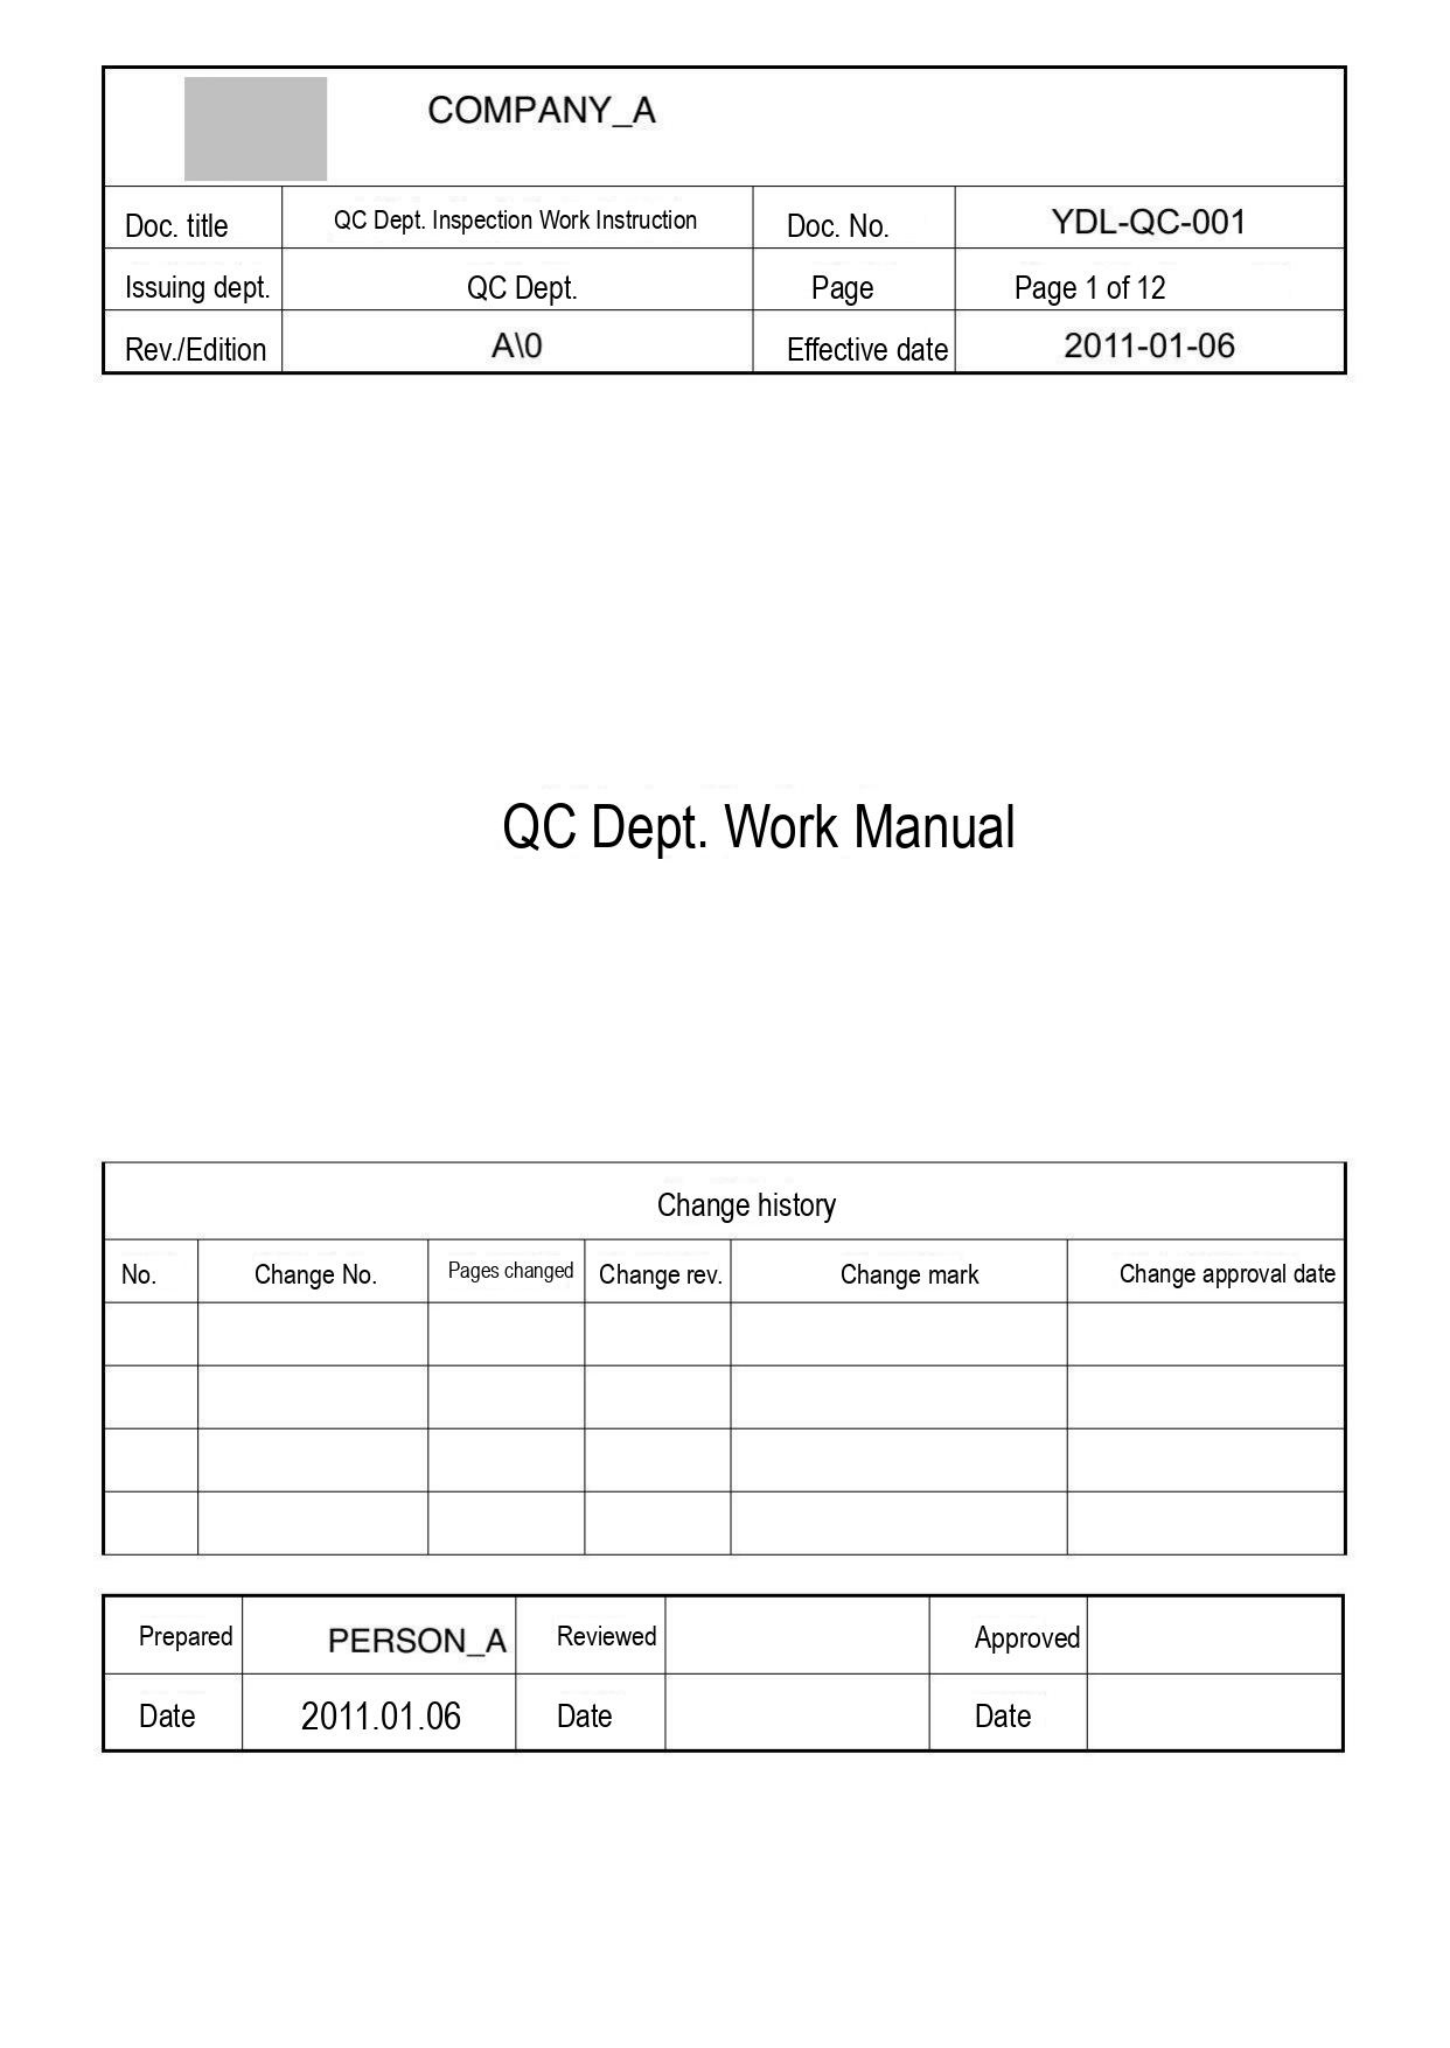COMPANY_A

| Doc. title | QC Dept. Inspection Work Instruction | Doc. No. | YDL-QC-001 |
|---|---|---|---|
| Issuing dept. | QC Dept. | Page | Page 1 of 12 |
| Rev./Edition | A\0 | Effective date | 2011-01-06 |

QC Dept. Work Manual

Change history

| No. | Change No. | Pages changed | Change rev. | Change mark | Change approval date |
|---|---|---|---|---|---|
| | | | | | |
| | | | | | |
| | | | | | |
| | | | | | |

| Prepared | PERSON_A | Reviewed | | Approved | |
|---|---|---|---|---|---|
| Date | 2011.01.06 | Date | | Date | |
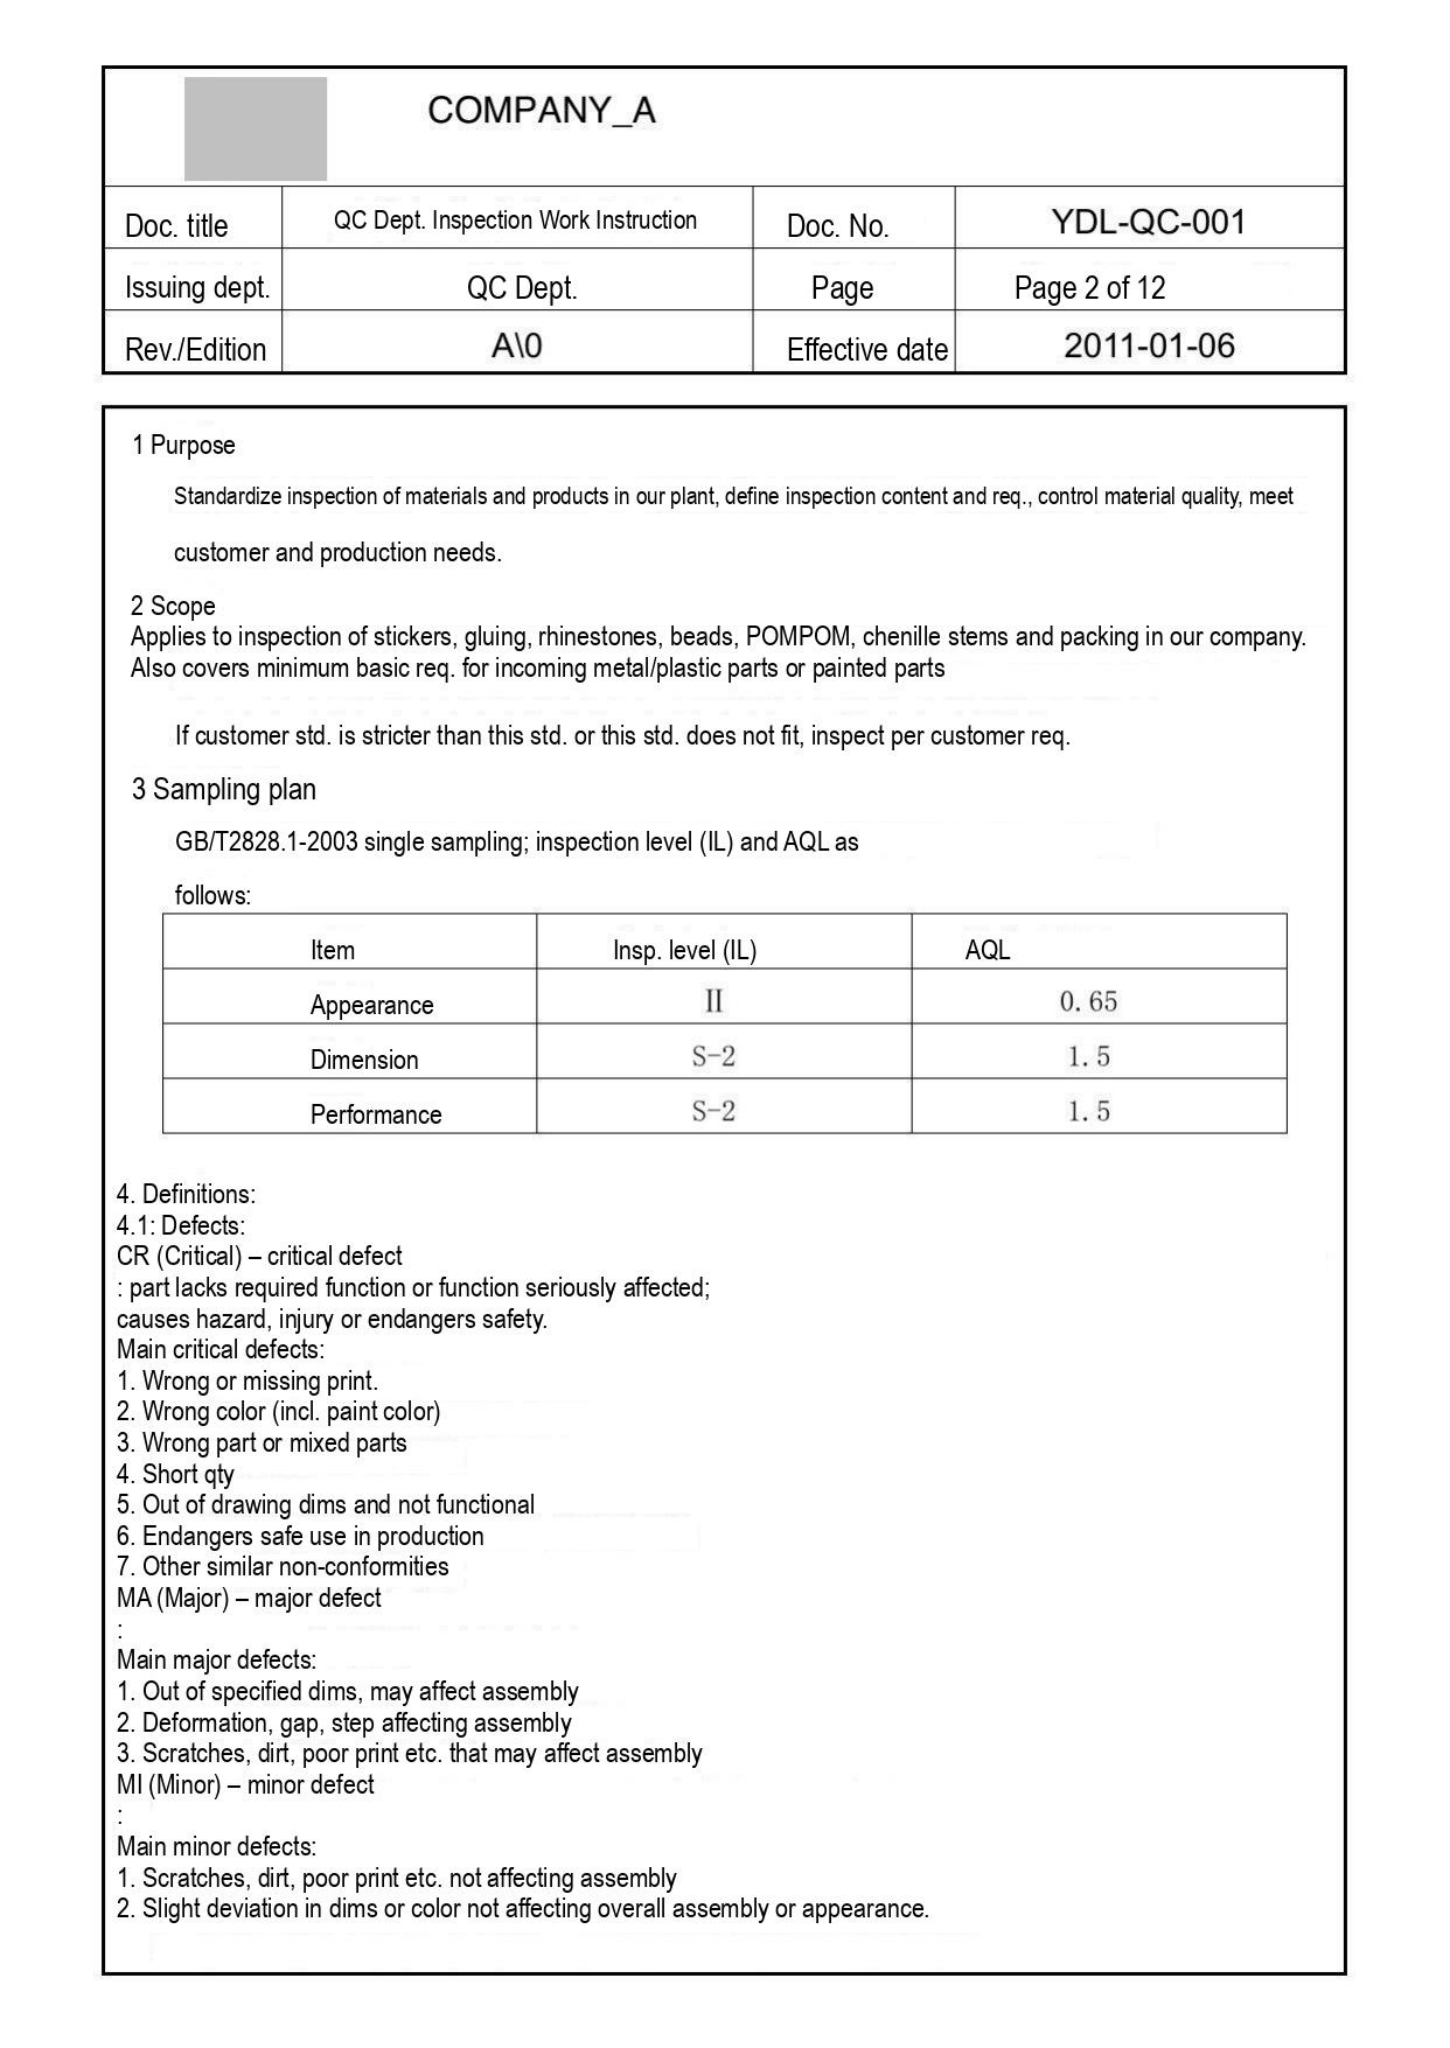COMPANY_A

| Doc. title | QC Dept. Inspection Work Instruction | Doc. No. | YDL-QC-001 |
|---|---|---|---|
| Issuing dept. | QC Dept. | Page | Page 2 of 12 |
| Rev./Edition | A\0 | Effective date | 2011-01-06 |

1 Purpose

Standardize inspection of materials and products in our plant, define inspection content and req., control material quality, meet customer and production needs.

2 Scope
Applies to inspection of stickers, gluing, rhinestones, beads, POMPOM, chenille stems and packing in our company. Also covers minimum basic req. for incoming metal/plastic parts or painted parts

If customer std. is stricter than this std. or this std. does not fit, inspect per customer req.

3 Sampling plan

GB/T2828.1-2003 single sampling; inspection level (IL) and AQL as follows:

| Item | Insp. level (IL) | AQL |
|---|---|---|
| Appearance | II | 0. 65 |
| Dimension | S-2 | 1. 5 |
| Performance | S-2 | 1. 5 |

4. Definitions:
4.1: Defects:
CR (Critical) – critical defect
: part lacks required function or function seriously affected;
causes hazard, injury or endangers safety.
Main critical defects:
1. Wrong or missing print.
2. Wrong color (incl. paint color)
3. Wrong part or mixed parts
4. Short qty
5. Out of drawing dims and not functional
6. Endangers safe use in production
7. Other similar non-conformities
MA (Major) – major defect
:
Main major defects:
1. Out of specified dims, may affect assembly
2. Deformation, gap, step affecting assembly
3. Scratches, dirt, poor print etc. that may affect assembly
MI (Minor) – minor defect
:
Main minor defects:
1. Scratches, dirt, poor print etc. not affecting assembly
2. Slight deviation in dims or color not affecting overall assembly or appearance.
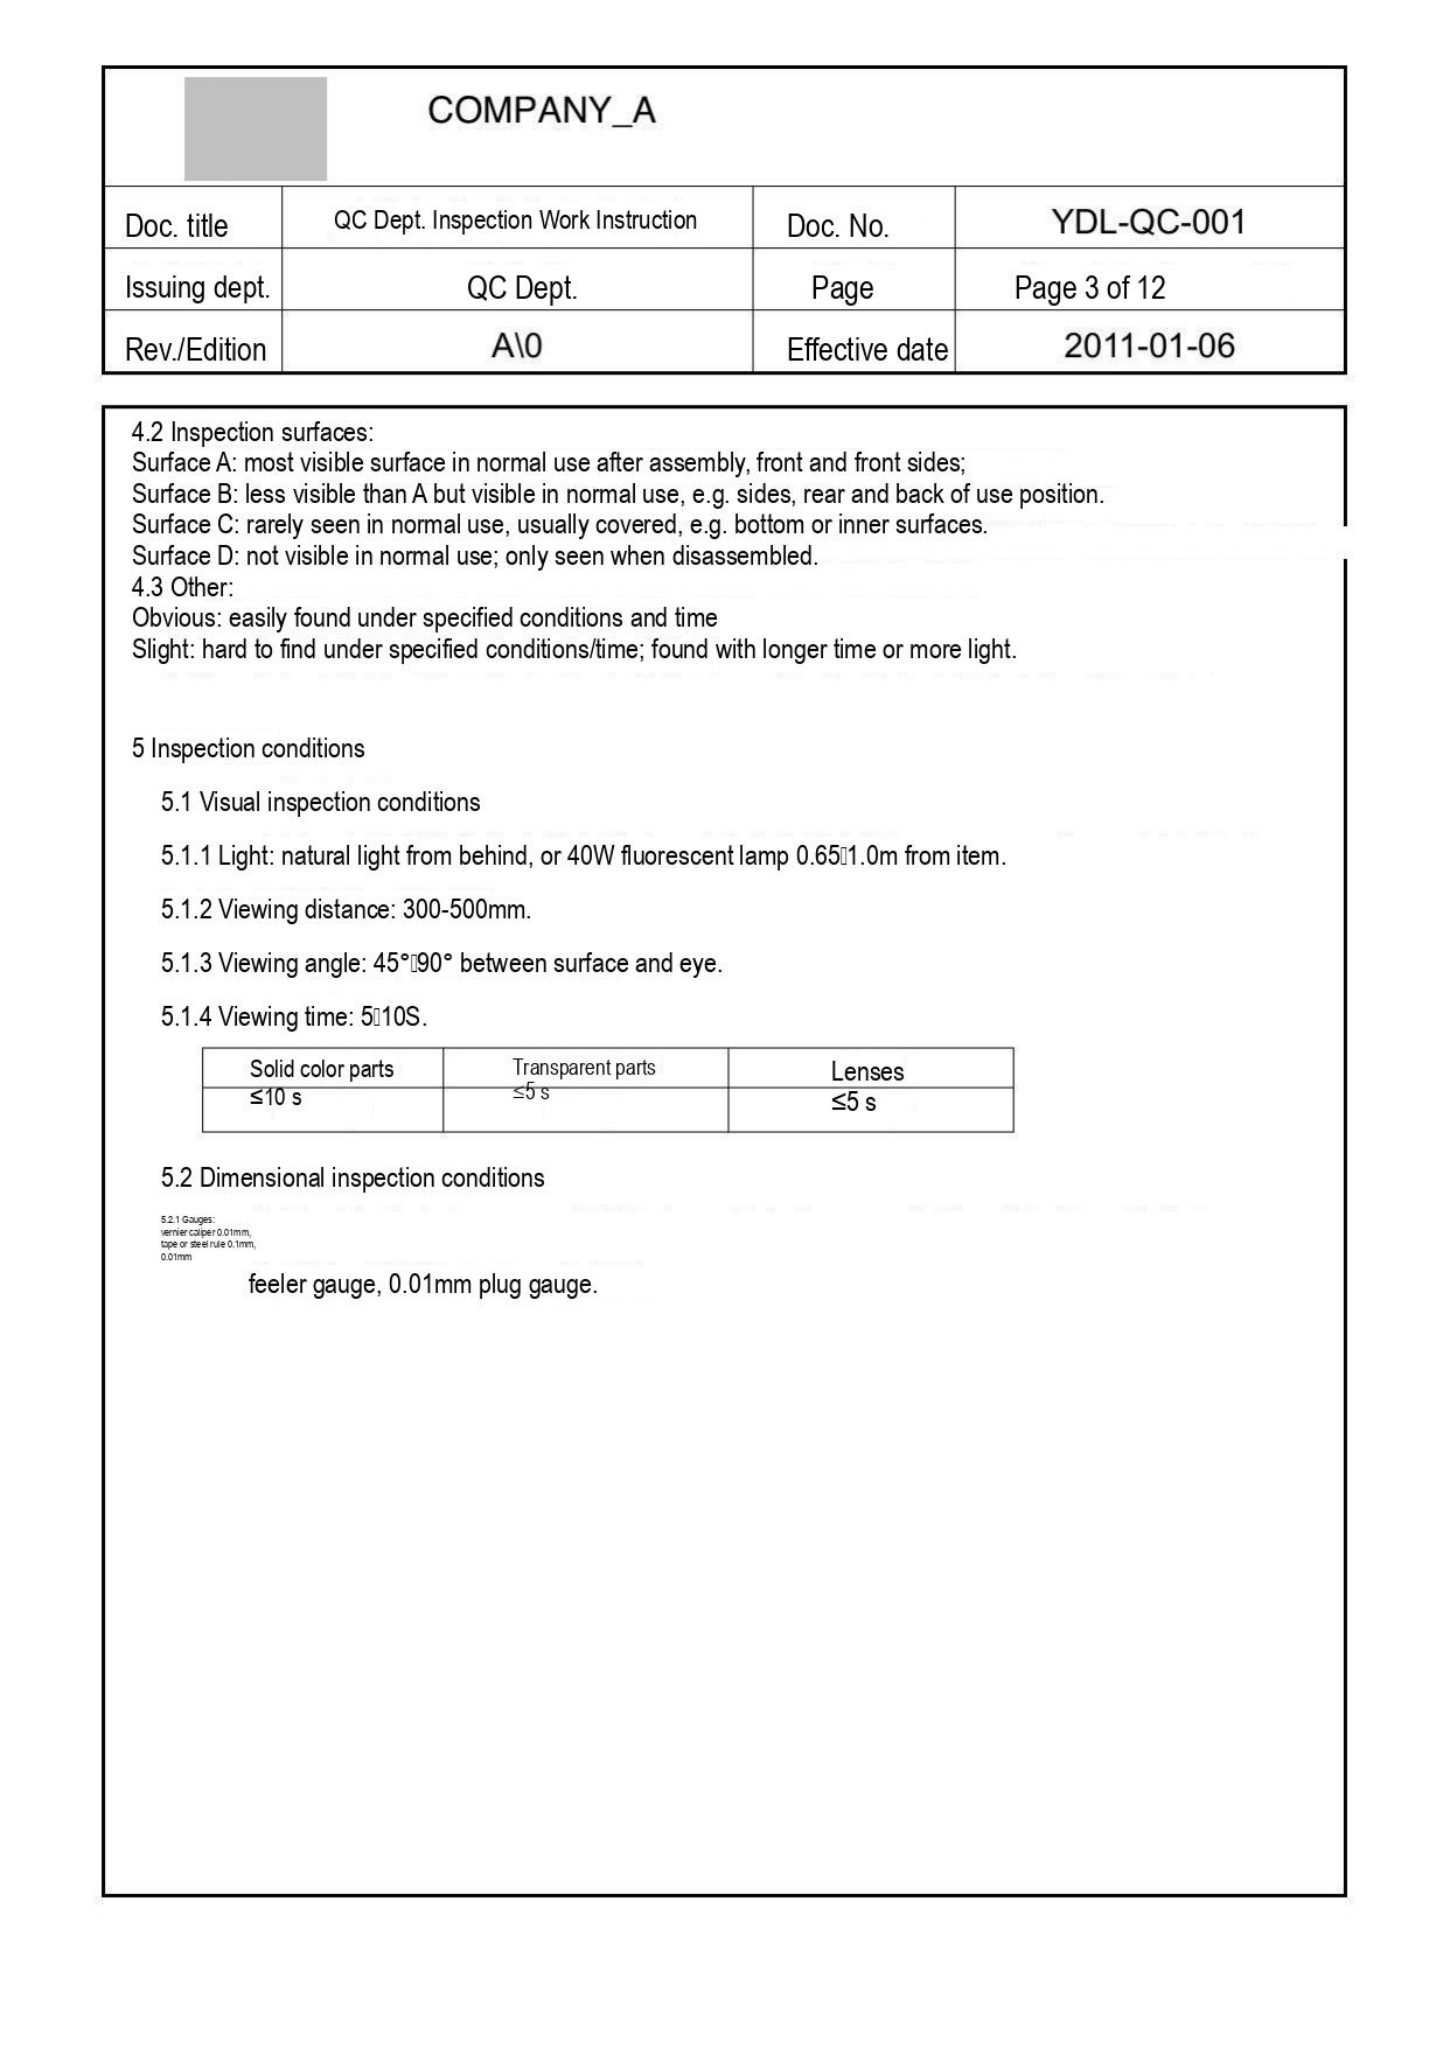COMPANY_A

| Doc. title | QC Dept. Inspection Work Instruction | Doc. No. | YDL-QC-001 |
|---|---|---|---|
| Issuing dept. | QC Dept. | Page | Page 3 of 12 |
| Rev./Edition | A\0 | Effective date | 2011-01-06 |

4.2 Inspection surfaces:
Surface A: most visible surface in normal use after assembly, front and front sides;
Surface B: less visible than A but visible in normal use, e.g. sides, rear and back of use position.
Surface C: rarely seen in normal use, usually covered, e.g. bottom or inner surfaces.
Surface D: not visible in normal use; only seen when disassembled.
4.3 Other:
Obvious: easily found under specified conditions and time
Slight: hard to find under specified conditions/time; found with longer time or more light.

5 Inspection conditions

5.1 Visual inspection conditions

5.1.1 Light: natural light from behind, or 40W fluorescent lamp 0.65 1.0m from item.

5.1.2 Viewing distance: 300-500mm.

5.1.3 Viewing angle: 45° 90° between surface and eye.

5.1.4 Viewing time: 5 10S.

| Solid color parts | Transparent parts | Lenses |
|---|---|---|
| ≤10 s | ≤5 s | ≤5 s |

5.2 Dimensional inspection conditions

5.2.1 Gauges:
vernier caliper 0.01mm,
tape or steel rule 0.1mm,
0.01mm

feeler gauge, 0.01mm plug gauge.
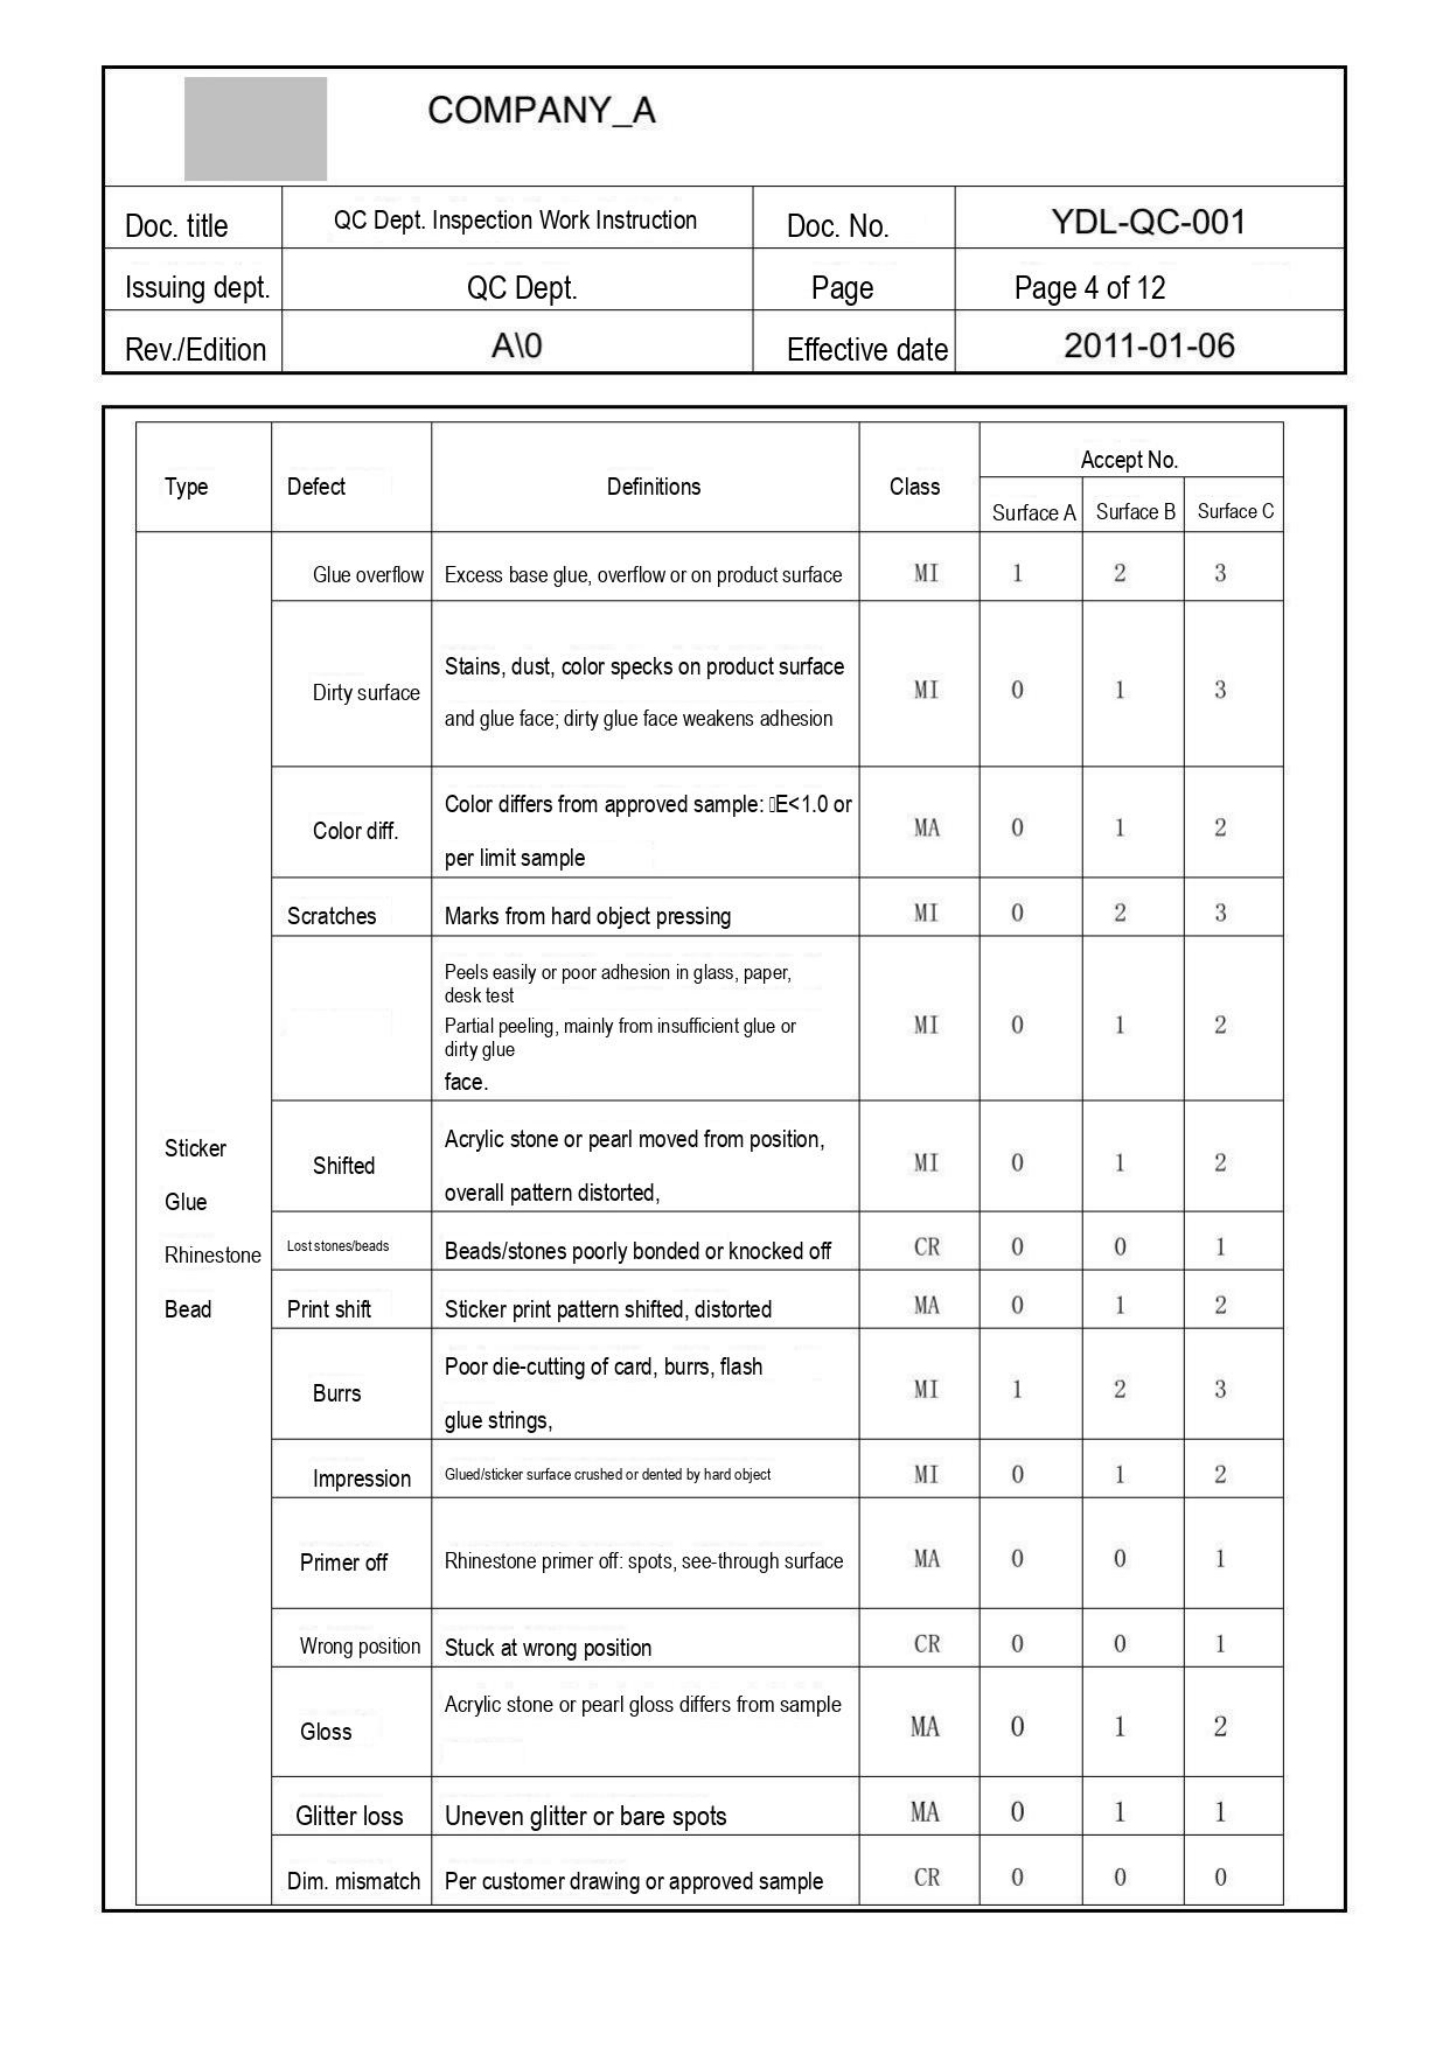COMPANY_A

| Doc. title | QC Dept. Inspection Work Instruction | Doc. No. | YDL-QC-001 |
|---|---|---|---|
| Issuing dept. | QC Dept. | Page | Page 4 of 12 |
| Rev./Edition | A\0 | Effective date | 2011-01-06 |

| Type | Defect | Definitions | Class | Accept No. Surface A | Accept No. Surface B | Accept No. Surface C |
|---|---|---|---|---|---|---|
| Sticker Glue Rhinestone Bead | Glue overflow | Excess base glue, overflow or on product surface | MI | 1 | 2 | 3 |
| | Dirty surface | Stains, dust, color specks on product surface and glue face; dirty glue face weakens adhesion | MI | 0 | 1 | 3 |
| | Color diff. | Color differs from approved sample: E<1.0 or per limit sample | MA | 0 | 1 | 2 |
| | Scratches | Marks from hard object pressing | MI | 0 | 2 | 3 |
| | | Peels easily or poor adhesion in glass, paper, desk test Partial peeling, mainly from insufficient glue or dirty glue face. | MI | 0 | 1 | 2 |
| | Shifted | Acrylic stone or pearl moved from position, overall pattern distorted, | MI | 0 | 1 | 2 |
| | Lost stones/beads | Beads/stones poorly bonded or knocked off | CR | 0 | 0 | 1 |
| | Print shift | Sticker print pattern shifted, distorted | MA | 0 | 1 | 2 |
| | Burrs | Poor die-cutting of card, burrs, flash glue strings, | MI | 1 | 2 | 3 |
| | Impression | Glued/sticker surface crushed or dented by hard object | MI | 0 | 1 | 2 |
| | Primer off | Rhinestone primer off: spots, see-through surface | MA | 0 | 0 | 1 |
| | Wrong position | Stuck at wrong position | CR | 0 | 0 | 1 |
| | Gloss | Acrylic stone or pearl gloss differs from sample | MA | 0 | 1 | 2 |
| | Glitter loss | Uneven glitter or bare spots | MA | 0 | 1 | 1 |
| | Dim. mismatch | Per customer drawing or approved sample | CR | 0 | 0 | 0 |
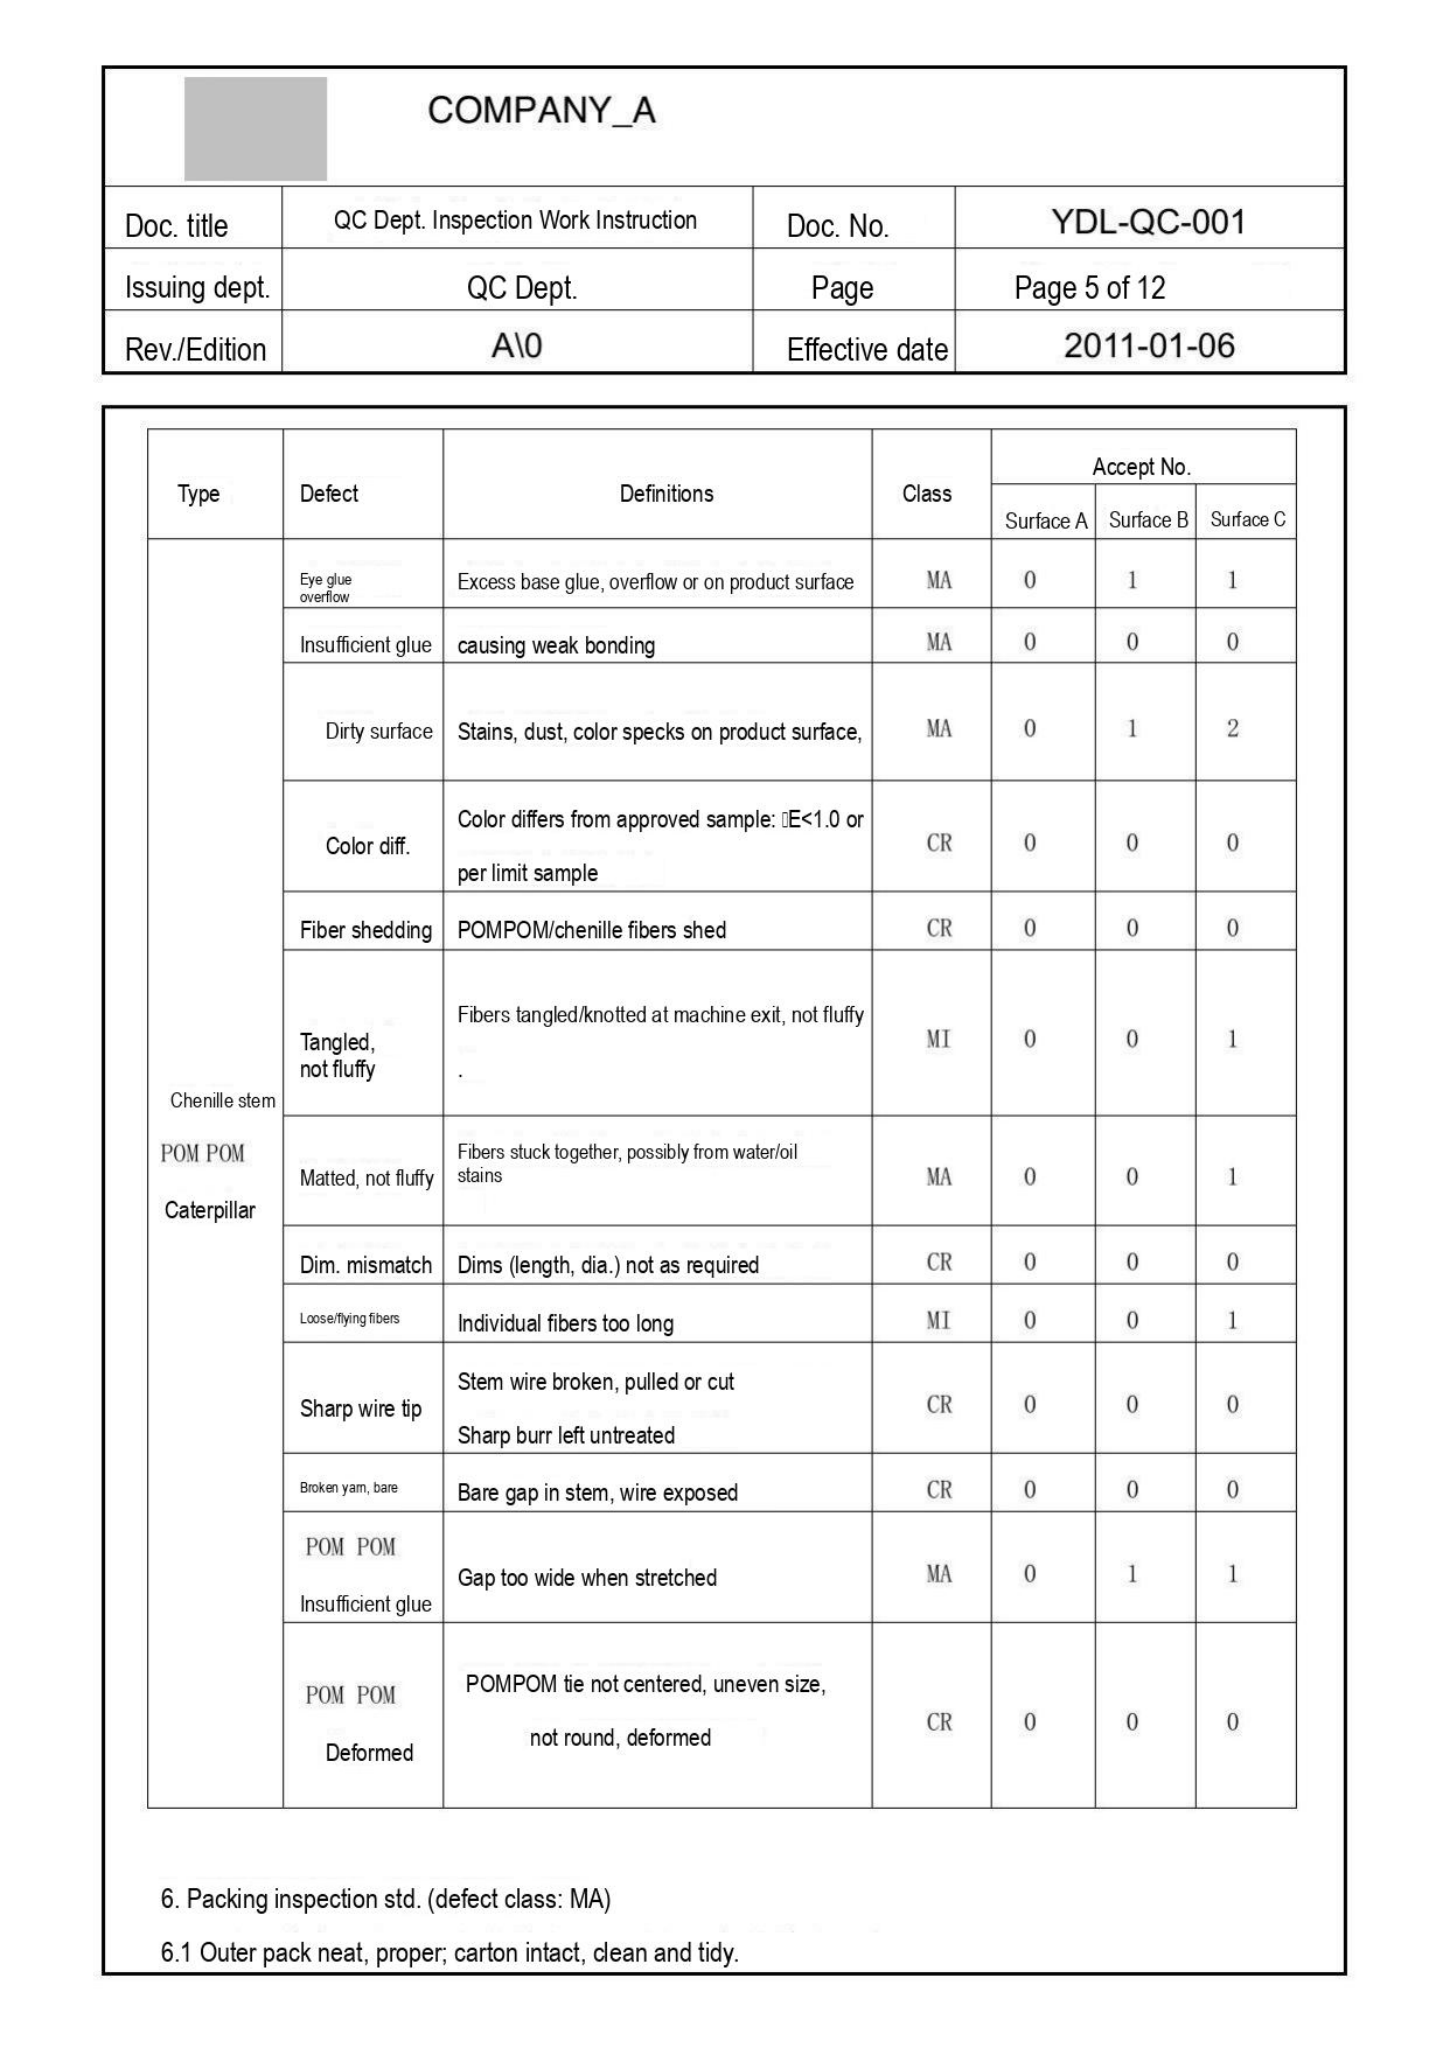COMPANY_A

| Doc. title | QC Dept. Inspection Work Instruction | Doc. No. | YDL-QC-001 |
|---|---|---|---|
| Issuing dept. | QC Dept. | Page | Page 5 of 12 |
| Rev./Edition | A\0 | Effective date | 2011-01-06 |

| Type | Defect | Definitions | Class | Accept No. Surface A | Accept No. Surface B | Accept No. Surface C |
|---|---|---|---|---|---|---|
| Chenille stem POM POM Caterpillar | Eye glue overflow | Excess base glue, overflow or on product surface | MA | 0 | 1 | 1 |
| | Insufficient glue | causing weak bonding | MA | 0 | 0 | 0 |
| | Dirty surface | Stains, dust, color specks on product surface, | MA | 0 | 1 | 2 |
| | Color diff. | Color differs from approved sample: E<1.0 or per limit sample | CR | 0 | 0 | 0 |
| | Fiber shedding | POMPOM/chenille fibers shed | CR | 0 | 0 | 0 |
| | Tangled, not fluffy | Fibers tangled/knotted at machine exit, not fluffy . | MI | 0 | 0 | 1 |
| | Matted, not fluffy | Fibers stuck together, possibly from water/oil stains | MA | 0 | 0 | 1 |
| | Dim. mismatch | Dims (length, dia.) not as required | CR | 0 | 0 | 0 |
| | Loose/flying fibers | Individual fibers too long | MI | 0 | 0 | 1 |
| | Sharp wire tip | Stem wire broken, pulled or cut Sharp burr left untreated | CR | 0 | 0 | 0 |
| | Broken yarn, bare | Bare gap in stem, wire exposed | CR | 0 | 0 | 0 |
| | POM POM Insufficient glue | Gap too wide when stretched | MA | 0 | 1 | 1 |
| | POM POM Deformed | POMPOM tie not centered, uneven size, not round, deformed | CR | 0 | 0 | 0 |

6. Packing inspection std. (defect class: MA)

6.1 Outer pack neat, proper; carton intact, clean and tidy.
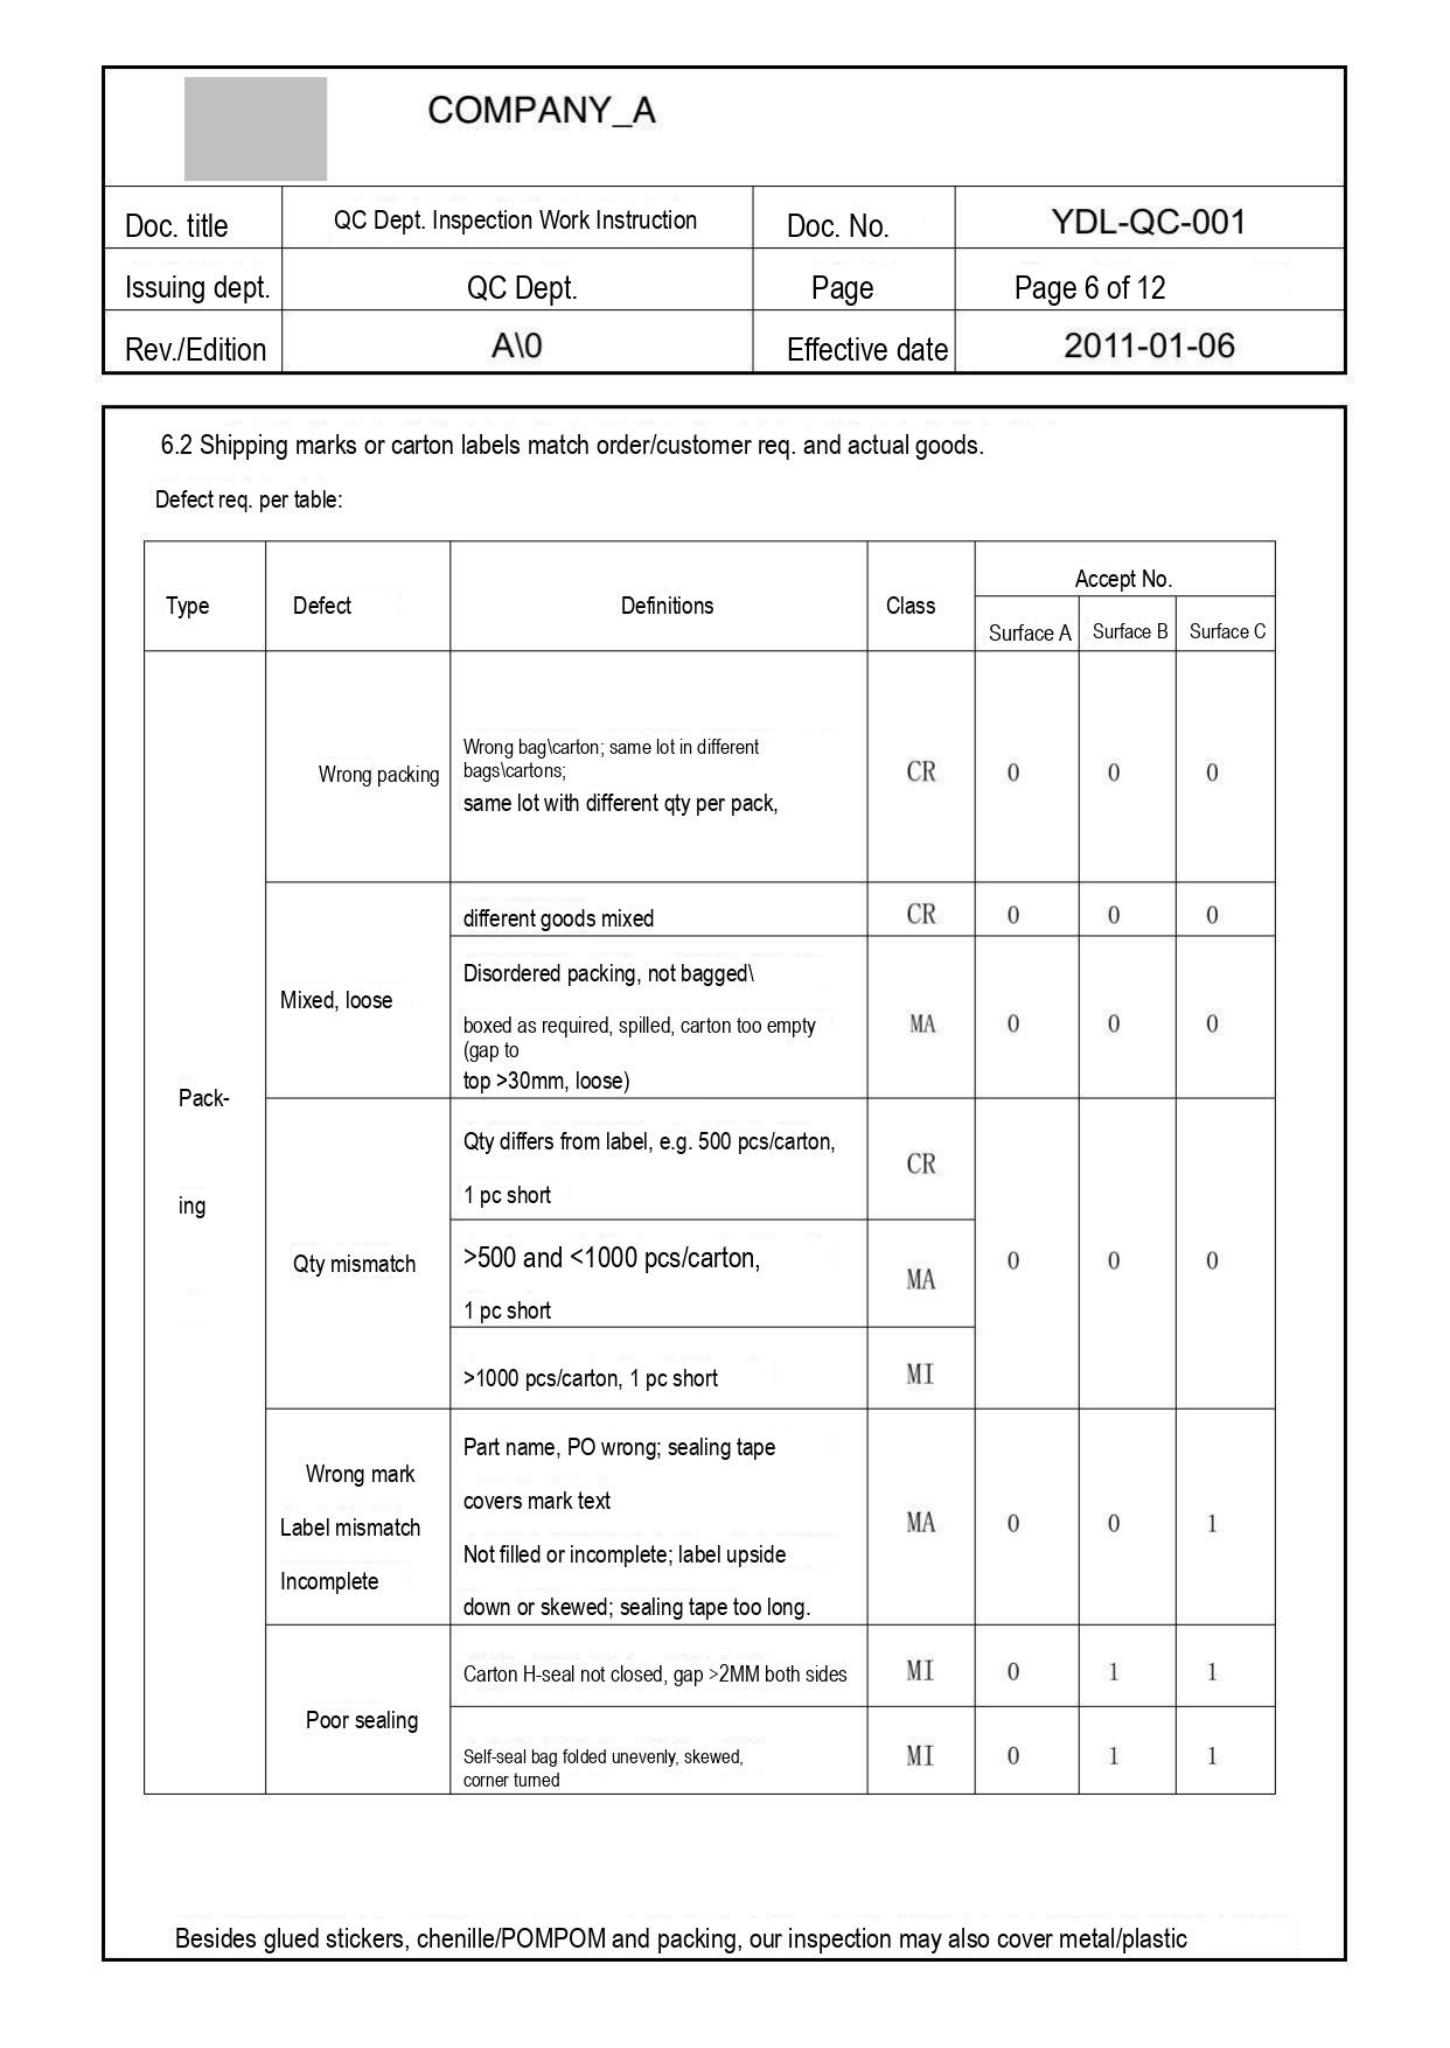COMPANY_A

| Doc. title | QC Dept. Inspection Work Instruction | Doc. No. | YDL-QC-001 |
|---|---|---|---|
| Issuing dept. | QC Dept. | Page | Page 6 of 12 |
| Rev./Edition | A\0 | Effective date | 2011-01-06 |

6.2 Shipping marks or carton labels match order/customer req. and actual goods.

Defect req. per table:

| Type | Defect | Definitions | Class | Accept No. Surface A | Accept No. Surface B | Accept No. Surface C |
|---|---|---|---|---|---|---|
| Pack-ing | Wrong packing | Wrong bag\carton; same lot in different bags\cartons; same lot with different qty per pack, | CR | 0 | 0 | 0 |
| | Mixed, loose | different goods mixed | CR | 0 | 0 | 0 |
| | | Disordered packing, not bagged\ boxed as required, spilled, carton too empty (gap to top >30mm, loose) | MA | 0 | 0 | 0 |
| | Qty mismatch | Qty differs from label, e.g. 500 pcs/carton, 1 pc short | CR | 0 | 0 | 0 |
| | | >500 and <1000 pcs/carton, 1 pc short | MA | | | |
| | | >1000 pcs/carton, 1 pc short | MI | | | |
| | Wrong mark Label mismatch Incomplete | Part name, PO wrong; sealing tape covers mark text Not filled or incomplete; label upside down or skewed; sealing tape too long. | MA | 0 | 0 | 1 |
| | Poor sealing | Carton H-seal not closed, gap >2MM both sides | MI | 0 | 1 | 1 |
| | | Self-seal bag folded unevenly, skewed, corner turned | MI | 0 | 1 | 1 |

Besides glued stickers, chenille/POMPOM and packing, our inspection may also cover metal/plastic
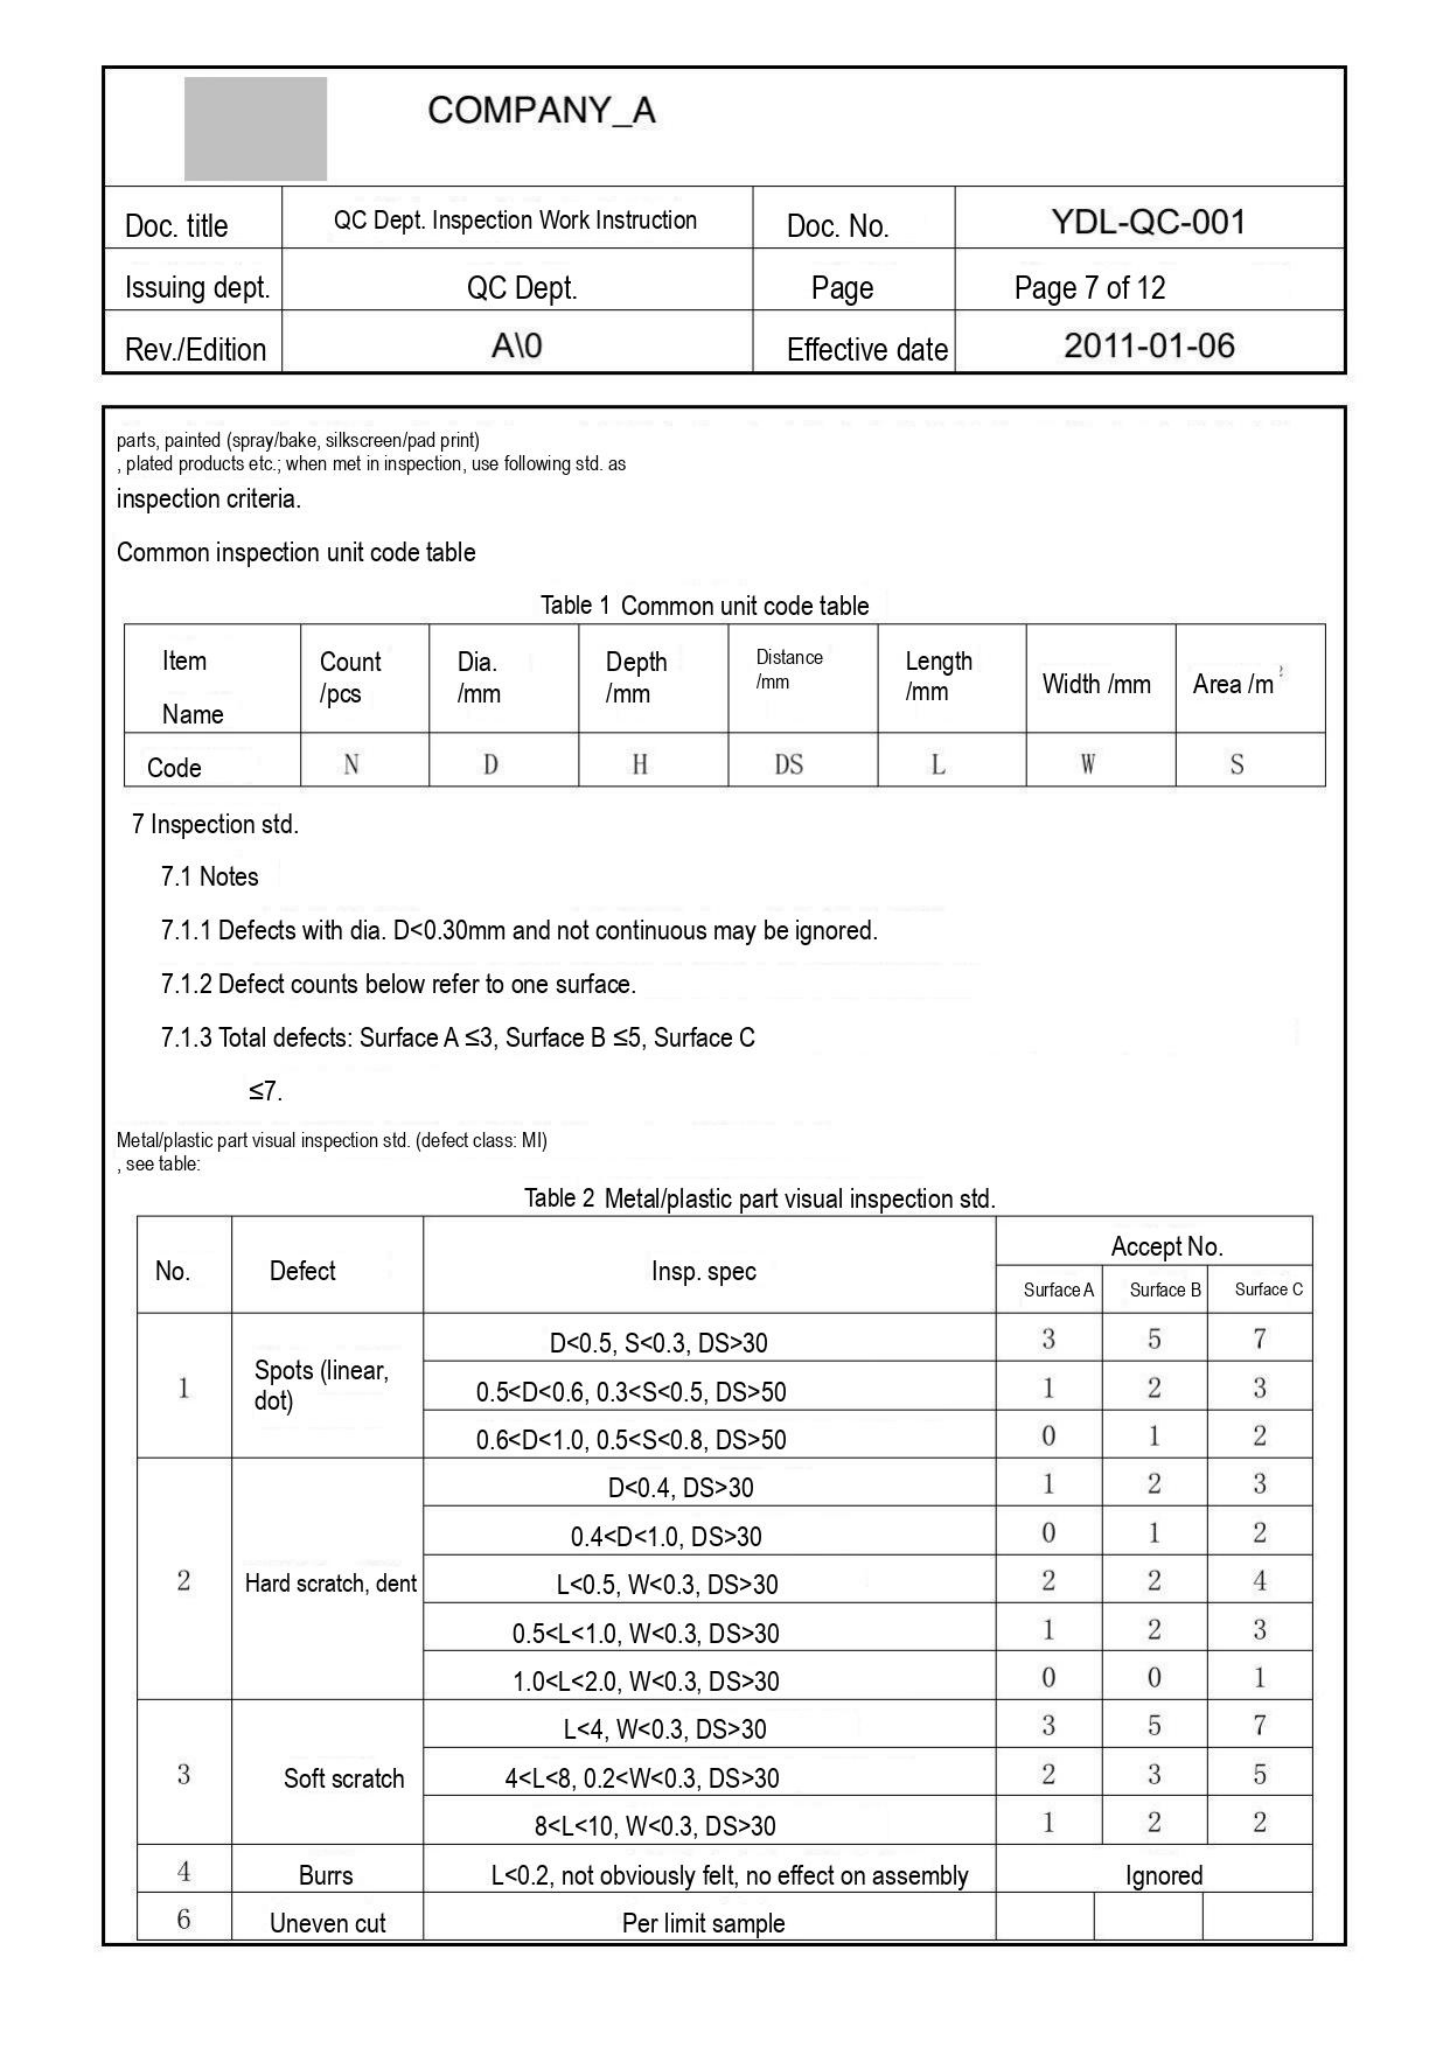COMPANY_A

| Doc. title | QC Dept. Inspection Work Instruction | Doc. No. | YDL-QC-001 |
|---|---|---|---|
| Issuing dept. | QC Dept. | Page | Page 7 of 12 |
| Rev./Edition | A\0 | Effective date | 2011-01-06 |

parts, painted (spray/bake, silkscreen/pad print)
, plated products etc.; when met in inspection, use following std. as
inspection criteria.

Common inspection unit code table

Table 1 Common unit code table

| Item Name | Count /pcs | Dia. /mm | Depth /mm | Distance /mm | Length /mm | Width /mm | Area /m² |
|---|---|---|---|---|---|---|---|
| Code | N | D | H | DS | L | W | S |

7 Inspection std.

7.1 Notes

7.1.1 Defects with dia. D<0.30mm and not continuous may be ignored.

7.1.2 Defect counts below refer to one surface.

7.1.3 Total defects: Surface A ≤3, Surface B ≤5, Surface C ≤7.

Metal/plastic part visual inspection std. (defect class: MI)
, see table:

Table 2 Metal/plastic part visual inspection std.

| No. | Defect | Insp. spec | Accept No. Surface A | Accept No. Surface B | Accept No. Surface C |
|---|---|---|---|---|---|
| 1 | Spots (linear, dot) | D<0.5, S<0.3, DS>30 | 3 | 5 | 7 |
| | | 0.5<D<0.6, 0.3<S<0.5, DS>50 | 1 | 2 | 3 |
| | | 0.6<D<1.0, 0.5<S<0.8, DS>50 | 0 | 1 | 2 |
| 2 | Hard scratch, dent | D<0.4, DS>30 | 1 | 2 | 3 |
| | | 0.4<D<1.0, DS>30 | 0 | 1 | 2 |
| | | L<0.5, W<0.3, DS>30 | 2 | 2 | 4 |
| | | 0.5<L<1.0, W<0.3, DS>30 | 1 | 2 | 3 |
| | | 1.0<L<2.0, W<0.3, DS>30 | 0 | 0 | 1 |
| 3 | Soft scratch | L<4, W<0.3, DS>30 | 3 | 5 | 7 |
| | | 4<L<8, 0.2<W<0.3, DS>30 | 2 | 3 | 5 |
| | | 8<L<10, W<0.3, DS>30 | 1 | 2 | 2 |
| 4 | Burrs | L<0.2, not obviously felt, no effect on assembly | Ignored | | |
| 6 | Uneven cut | Per limit sample | | | |